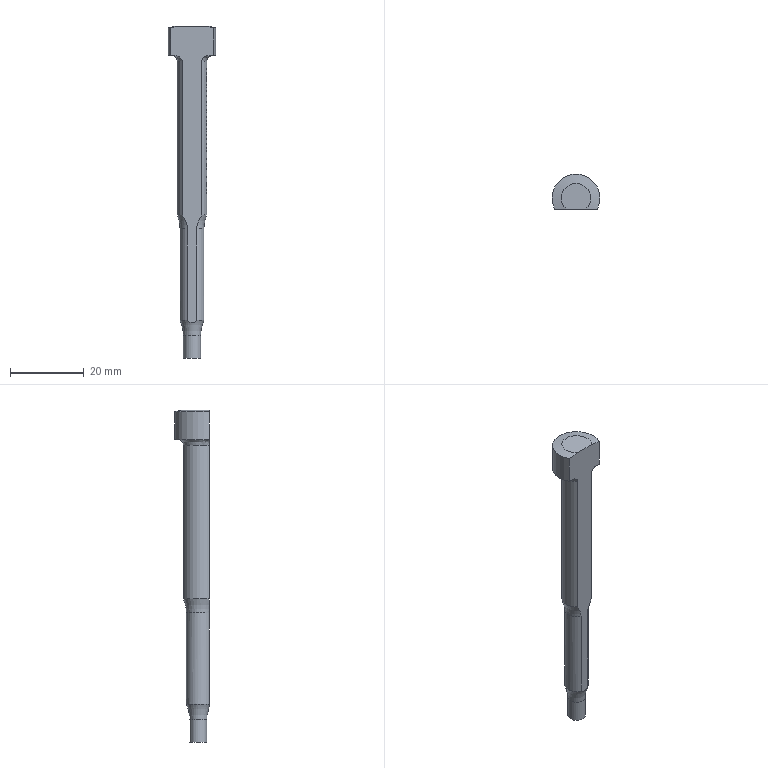Part | NX | features MI_APTWA_0170 2 | 1 solid | 471 faces | box 13 x 9.5 x 90 mm | volume 3991 mm3 | plane 286 | cylinder 181 | torus 2 | spline 1 | cone 1 | commonest cylinder face diameters 7.8 x36 8 x20 0.827 x5 0.462 x4 0.578 x4 0.605 x4